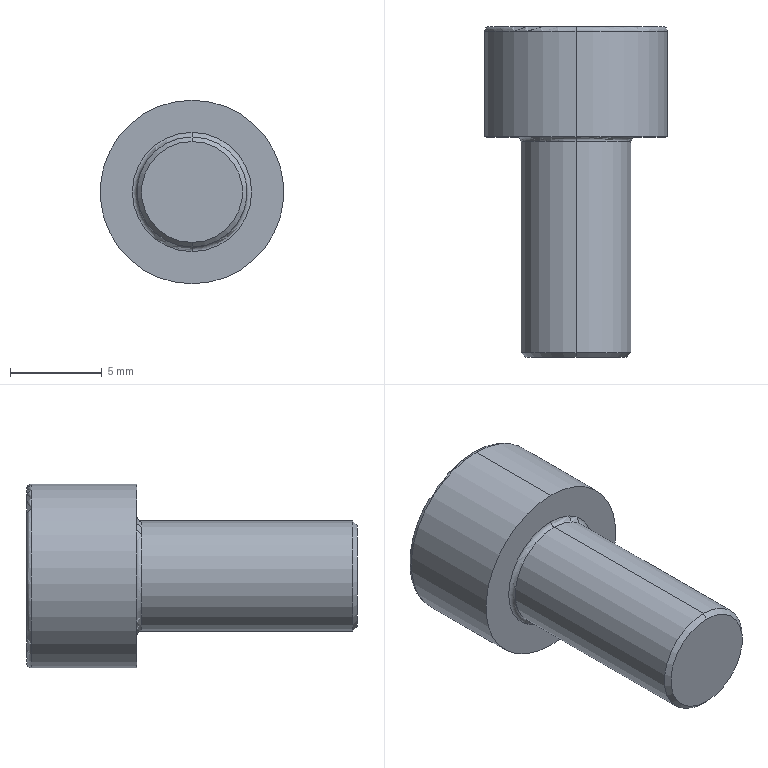Part | STEP file | 1 solid | 20 faces | box 10 x 18 x 10 mm | volume 744.847 mm3 | plane 10 | torus 4 | cylinder 4 | cone 2 | commonest cylinder face diameters 6 x2 10 x2
STEP:
#1=CARTESIAN_POINT('',(0.,-12.,-2.75));
#2=VERTEX_POINT('',#1);
#3=CARTESIAN_POINT('',(0.,-12.,2.75));
#4=VERTEX_POINT('',#3);
#5=CARTESIAN_POINT('',(0.,-12.,0.));
#6=DIRECTION('',(0.,-1.,0.));
#7=DIRECTION('',(0.,0.,-1.));
#8=AXIS2_PLACEMENT_3D('',#5,#6,#7);
#9=CIRCLE('',#8,2.75);
#10=EDGE_CURVE('',#2,#4,#9,.T.);
#11=ORIENTED_EDGE('',*,*,#10,.F.);
#12=CARTESIAN_POINT('',(0.,-11.75,-3.));
#13=VERTEX_POINT('',#12);
#14=CARTESIAN_POINT('',(0.,-12.,-2.75));
#15=DIRECTION('',(0.,0.7071,-0.7071));
#16=VECTOR('',#15,1000.);
#17=LINE('',#14,#16);
#18=EDGE_CURVE('',#2,#13,#17,.T.);
#19=ORIENTED_EDGE('',*,*,#18,.T.);
#20=CARTESIAN_POINT('',(0.,-11.75,3.));
#21=VERTEX_POINT('',#20);
#22=CARTESIAN_POINT('',(0.,-11.75,0.));
#23=DIRECTION('',(0.,1.,0.));
#24=DIRECTION('',(0.,0.,-1.));
#25=AXIS2_PLACEMENT_3D('',#22,#23,#24);
#26=CIRCLE('',#25,3.);
#27=EDGE_CURVE('',#21,#13,#26,.T.);
#28=ORIENTED_EDGE('',*,*,#27,.F.);
#29=CARTESIAN_POINT('',(0.,-12.,2.75));
#30=DIRECTION('',(0.,0.7071,0.7071));
#31=VECTOR('',#30,1000.);
#32=LINE('',#29,#31);
#33=EDGE_CURVE('',#4,#21,#32,.T.);
#34=ORIENTED_EDGE('',*,*,#33,.F.);
#35=EDGE_LOOP('',(#11,#19,#28,#34));
#36=FACE_OUTER_BOUND('',#35,.T.);
#37=CARTESIAN_POINT('',(0.,-12.,0.));
#38=DIRECTION('',(0.,1.,0.));
#39=DIRECTION('',(0.,0.,1.));
#40=AXIS2_PLACEMENT_3D('',#37,#38,#39);
#41=CONICAL_SURFACE('',#40,2.75,0.7854);
#42=ADVANCED_FACE('',(#36),#41,.T.);
#43=CARTESIAN_POINT('',(0.,5.75,-5.));
#44=VERTEX_POINT('',#43);
#45=CARTESIAN_POINT('',(0.,5.75,5.));
#46=VERTEX_POINT('',#45);
#47=CARTESIAN_POINT('',(0.,5.75,0.));
#48=DIRECTION('',(0.,-1.,0.));
#49=DIRECTION('',(0.,0.,1.));
#50=AXIS2_PLACEMENT_3D('',#47,#48,#49);
#51=CIRCLE('',#50,5.);
#52=EDGE_CURVE('',#44,#46,#51,.T.);
#53=ORIENTED_EDGE('',*,*,#52,.F.);
#54=CARTESIAN_POINT('',(0.,6.,-4.75));
#55=VERTEX_POINT('',#54);
#56=CARTESIAN_POINT('',(0.,5.75,-4.75));
#57=DIRECTION('',(1.,0.,0.));
#58=DIRECTION('',(0.,0.,-1.));
#59=AXIS2_PLACEMENT_3D('',#56,#57,#58);
#60=CIRCLE('',#59,0.25);
#61=EDGE_CURVE('',#44,#55,#60,.T.);
#62=ORIENTED_EDGE('',*,*,#61,.T.);
#63=CARTESIAN_POINT('',(0.,6.,4.75));
#64=VERTEX_POINT('',#63);
#65=CARTESIAN_POINT('',(0.,6.,0.));
#66=DIRECTION('',(0.,1.,0.));
#67=DIRECTION('',(0.,0.,1.));
#68=AXIS2_PLACEMENT_3D('',#65,#66,#67);
#69=CIRCLE('',#68,4.75);
#70=EDGE_CURVE('',#64,#55,#69,.T.);
#71=ORIENTED_EDGE('',*,*,#70,.F.);
#72=CARTESIAN_POINT('',(0.,5.75,4.75));
#73=DIRECTION('',(-1.,0.,0.));
#74=DIRECTION('',(0.,0.,1.));
#75=AXIS2_PLACEMENT_3D('',#72,#73,#74);
#76=CIRCLE('',#75,0.25);
#77=EDGE_CURVE('',#46,#64,#76,.T.);
#78=ORIENTED_EDGE('',*,*,#77,.F.);
#79=EDGE_LOOP('',(#53,#62,#71,#78));
#80=FACE_OUTER_BOUND('',#79,.T.);
#81=CARTESIAN_POINT('',(0.,5.75,0.));
#82=DIRECTION('',(0.,1.,0.));
#83=DIRECTION('',(0.,0.,1.));
#84=AXIS2_PLACEMENT_3D('',#81,#82,#83);
#85=TOROIDAL_SURFACE('',#84,4.75,0.25);
#86=ADVANCED_FACE('',(#80),#85,.T.);
#87=CARTESIAN_POINT('',(0.,-0.25,3.));
#88=VERTEX_POINT('',#87);
#89=CARTESIAN_POINT('',(0.,-0.25,-3.));
#90=VERTEX_POINT('',#89);
#91=CARTESIAN_POINT('',(0.,-0.25,0.));
#92=DIRECTION('',(0.,-1.,0.));
#93=DIRECTION('',(0.,0.,-1.));
#94=AXIS2_PLACEMENT_3D('',#91,#92,#93);
#95=CIRCLE('',#94,3.);
#96=EDGE_CURVE('',#88,#90,#95,.T.);
#97=ORIENTED_EDGE('',*,*,#96,.F.);
#98=CARTESIAN_POINT('',(0.,0.,3.25));
#99=VERTEX_POINT('',#98);
#100=CARTESIAN_POINT('',(0.,-0.25,3.25));
#101=DIRECTION('',(1.,0.,0.));
#102=DIRECTION('',(0.,0.,-1.));
#103=AXIS2_PLACEMENT_3D('',#100,#101,#102);
#104=CIRCLE('',#103,0.25);
#105=EDGE_CURVE('',#88,#99,#104,.T.);
#106=ORIENTED_EDGE('',*,*,#105,.T.);
#107=CARTESIAN_POINT('',(0.,0.,-3.25));
#108=VERTEX_POINT('',#107);
#109=CARTESIAN_POINT('',(0.,0.,0.));
#110=DIRECTION('',(0.,1.,0.));
#111=DIRECTION('',(0.,0.,-1.));
#112=AXIS2_PLACEMENT_3D('',#109,#110,#111);
#113=CIRCLE('',#112,3.25);
#114=EDGE_CURVE('',#108,#99,#113,.T.);
#115=ORIENTED_EDGE('',*,*,#114,.F.);
#116=CARTESIAN_POINT('',(0.,-0.25,-3.25));
#117=DIRECTION('',(-1.,0.,0.));
#118=DIRECTION('',(0.,0.,1.));
#119=AXIS2_PLACEMENT_3D('',#116,#117,#118);
#120=CIRCLE('',#119,0.25);
#121=EDGE_CURVE('',#90,#108,#120,.T.);
#122=ORIENTED_EDGE('',*,*,#121,.F.);
#123=EDGE_LOOP('',(#97,#106,#115,#122));
#124=FACE_OUTER_BOUND('',#123,.T.);
#125=CARTESIAN_POINT('',(0.,-0.25,0.));
#126=DIRECTION('',(0.,-1.,0.));
#127=DIRECTION('',(0.,0.,-1.));
#128=AXIS2_PLACEMENT_3D('',#125,#126,#127);
#129=TOROIDAL_SURFACE('',#128,3.25,0.25);
#130=ADVANCED_FACE('',(#124),#129,.F.);
#131=CARTESIAN_POINT('',(0.,-0.25,0.));
#132=DIRECTION('',(0.,-1.,0.));
#133=DIRECTION('',(0.,0.,-1.));
#134=AXIS2_PLACEMENT_3D('',#131,#132,#133);
#135=CIRCLE('',#134,3.);
#136=EDGE_CURVE('',#90,#88,#135,.T.);
#137=ORIENTED_EDGE('',*,*,#136,.T.);
#138=CARTESIAN_POINT('',(0.,0.,3.));
#139=DIRECTION('',(0.,-1.,0.));
#140=VECTOR('',#139,1000.);
#141=LINE('',#138,#140);
#142=EDGE_CURVE('',#88,#21,#141,.T.);
#143=ORIENTED_EDGE('',*,*,#142,.T.);
#144=ORIENTED_EDGE('',*,*,#27,.T.);
#145=CARTESIAN_POINT('',(0.,0.,-3.));
#146=DIRECTION('',(0.,-1.,0.));
#147=VECTOR('',#146,1000.);
#148=LINE('',#145,#147);
#149=EDGE_CURVE('',#90,#13,#148,.T.);
#150=ORIENTED_EDGE('',*,*,#149,.F.);
#151=EDGE_LOOP('',(#137,#143,#144,#150));
#152=FACE_OUTER_BOUND('',#151,.T.);
#153=CARTESIAN_POINT('',(0.,0.,0.));
#154=DIRECTION('',(0.,-1.,0.));
#155=DIRECTION('',(0.,0.,-1.));
#156=AXIS2_PLACEMENT_3D('',#153,#154,#155);
#157=CYLINDRICAL_SURFACE('',#156,3.);
#158=ADVANCED_FACE('',(#152),#157,.T.);
#159=ORIENTED_EDGE('',*,*,#52,.T.);
#160=CARTESIAN_POINT('',(0.,0.,5.));
#161=VERTEX_POINT('',#160);
#162=CARTESIAN_POINT('',(0.,0.,5.));
#163=DIRECTION('',(0.,-1.,0.));
#164=VECTOR('',#163,1000.);
#165=LINE('',#162,#164);
#166=EDGE_CURVE('',#46,#161,#165,.T.);
#167=ORIENTED_EDGE('',*,*,#166,.T.);
#168=CARTESIAN_POINT('',(0.,0.,-5.));
#169=VERTEX_POINT('',#168);
#170=CARTESIAN_POINT('',(0.,0.,0.));
#171=DIRECTION('',(0.,-1.,0.));
#172=DIRECTION('',(0.,0.,-1.));
#173=AXIS2_PLACEMENT_3D('',#170,#171,#172);
#174=CIRCLE('',#173,5.);
#175=EDGE_CURVE('',#169,#161,#174,.T.);
#176=ORIENTED_EDGE('',*,*,#175,.F.);
#177=CARTESIAN_POINT('',(0.,0.,-5.));
#178=DIRECTION('',(0.,-1.,0.));
#179=VECTOR('',#178,1000.);
#180=LINE('',#177,#179);
#181=EDGE_CURVE('',#44,#169,#180,.T.);
#182=ORIENTED_EDGE('',*,*,#181,.F.);
#183=EDGE_LOOP('',(#159,#167,#176,#182));
#184=FACE_OUTER_BOUND('',#183,.T.);
#185=CARTESIAN_POINT('',(0.,0.,0.));
#186=DIRECTION('',(0.,-1.,0.));
#187=DIRECTION('',(0.,0.,-1.));
#188=AXIS2_PLACEMENT_3D('',#185,#186,#187);
#189=CYLINDRICAL_SURFACE('',#188,5.);
#190=ADVANCED_FACE('',(#184),#189,.T.);
#191=ORIENTED_EDGE('',*,*,#70,.T.);
#192=CARTESIAN_POINT('',(0.,6.,0.));
#193=DIRECTION('',(0.,1.,0.));
#194=DIRECTION('',(0.,0.,1.));
#195=AXIS2_PLACEMENT_3D('',#192,#193,#194);
#196=CIRCLE('',#195,4.75);
#197=EDGE_CURVE('',#55,#64,#196,.T.);
#198=ORIENTED_EDGE('',*,*,#197,.T.);
#199=EDGE_LOOP('',(#191,#198));
#200=FACE_OUTER_BOUND('',#199,.T.);
#201=CARTESIAN_POINT('',(0.,6.,-2.887));
#202=VERTEX_POINT('',#201);
#203=CARTESIAN_POINT('',(-2.5,6.,-1.443));
#204=VERTEX_POINT('',#203);
#205=CARTESIAN_POINT('',(0.,6.,-2.887));
#206=DIRECTION('',(-0.866,0.,0.5));
#207=VECTOR('',#206,1000.);
#208=LINE('',#205,#207);
#209=EDGE_CURVE('',#202,#204,#208,.T.);
#210=ORIENTED_EDGE('',*,*,#209,.F.);
#211=CARTESIAN_POINT('',(2.5,6.,-1.443));
#212=VERTEX_POINT('',#211);
#213=CARTESIAN_POINT('',(2.5,6.,-1.443));
#214=DIRECTION('',(-0.866,0.,-0.5));
#215=VECTOR('',#214,1000.);
#216=LINE('',#213,#215);
#217=EDGE_CURVE('',#212,#202,#216,.T.);
#218=ORIENTED_EDGE('',*,*,#217,.F.);
#219=CARTESIAN_POINT('',(2.5,6.,1.443));
#220=VERTEX_POINT('',#219);
#221=CARTESIAN_POINT('',(2.5,6.,1.443));
#222=DIRECTION('',(0.,0.,-1.));
#223=VECTOR('',#222,1000.);
#224=LINE('',#221,#223);
#225=EDGE_CURVE('',#220,#212,#224,.T.);
#226=ORIENTED_EDGE('',*,*,#225,.F.);
#227=CARTESIAN_POINT('',(0.,6.,2.887));
#228=VERTEX_POINT('',#227);
#229=CARTESIAN_POINT('',(0.,6.,2.887));
#230=DIRECTION('',(0.866,0.,-0.5));
#231=VECTOR('',#230,1000.);
#232=LINE('',#229,#231);
#233=EDGE_CURVE('',#228,#220,#232,.T.);
#234=ORIENTED_EDGE('',*,*,#233,.F.);
#235=CARTESIAN_POINT('',(-2.5,6.,1.443));
#236=VERTEX_POINT('',#235);
#237=CARTESIAN_POINT('',(-2.5,6.,1.443));
#238=DIRECTION('',(0.866,0.,0.5));
#239=VECTOR('',#238,1000.);
#240=LINE('',#237,#239);
#241=EDGE_CURVE('',#236,#228,#240,.T.);
#242=ORIENTED_EDGE('',*,*,#241,.F.);
#243=CARTESIAN_POINT('',(-2.5,6.,-1.443));
#244=DIRECTION('',(0.,0.,1.));
#245=VECTOR('',#244,1000.);
#246=LINE('',#243,#245);
#247=EDGE_CURVE('',#204,#236,#246,.T.);
#248=ORIENTED_EDGE('',*,*,#247,.F.);
#249=EDGE_LOOP('',(#210,#218,#226,#234,#242,#248));
#250=FACE_BOUND('',#249,.T.);
#251=CARTESIAN_POINT('',(0.,6.,0.));
#252=DIRECTION('',(0.,1.,0.));
#253=DIRECTION('',(0.,0.,1.));
#254=AXIS2_PLACEMENT_3D('',#251,#252,#253);
#255=PLANE('',#254);
#256=ADVANCED_FACE('',(#200,#250),#255,.T.);
#257=ORIENTED_EDGE('',*,*,#166,.F.);
#258=CARTESIAN_POINT('',(0.,5.75,0.));
#259=DIRECTION('',(0.,-1.,0.));
#260=DIRECTION('',(0.,0.,1.));
#261=AXIS2_PLACEMENT_3D('',#258,#259,#260);
#262=CIRCLE('',#261,5.);
#263=EDGE_CURVE('',#46,#44,#262,.T.);
#264=ORIENTED_EDGE('',*,*,#263,.T.);
#265=ORIENTED_EDGE('',*,*,#181,.T.);
#266=CARTESIAN_POINT('',(0.,0.,0.));
#267=DIRECTION('',(0.,-1.,0.));
#268=DIRECTION('',(0.,0.,-1.));
#269=AXIS2_PLACEMENT_3D('',#266,#267,#268);
#270=CIRCLE('',#269,5.);
#271=EDGE_CURVE('',#161,#169,#270,.T.);
#272=ORIENTED_EDGE('',*,*,#271,.F.);
#273=EDGE_LOOP('',(#257,#264,#265,#272));
#274=FACE_OUTER_BOUND('',#273,.T.);
#275=CARTESIAN_POINT('',(0.,0.,0.));
#276=DIRECTION('',(0.,-1.,0.));
#277=DIRECTION('',(0.,0.,-1.));
#278=AXIS2_PLACEMENT_3D('',#275,#276,#277);
#279=CYLINDRICAL_SURFACE('',#278,5.);
#280=ADVANCED_FACE('',(#274),#279,.T.);
#281=ORIENTED_EDGE('',*,*,#114,.T.);
#282=CARTESIAN_POINT('',(0.,0.,0.));
#283=DIRECTION('',(0.,1.,0.));
#284=DIRECTION('',(0.,0.,-1.));
#285=AXIS2_PLACEMENT_3D('',#282,#283,#284);
#286=CIRCLE('',#285,3.25);
#287=EDGE_CURVE('',#99,#108,#286,.T.);
#288=ORIENTED_EDGE('',*,*,#287,.T.);
#289=EDGE_LOOP('',(#281,#288));
#290=FACE_BOUND('',#289,.T.);
#291=ORIENTED_EDGE('',*,*,#175,.T.);
#292=ORIENTED_EDGE('',*,*,#271,.T.);
#293=EDGE_LOOP('',(#291,#292));
#294=FACE_OUTER_BOUND('',#293,.T.);
#295=CARTESIAN_POINT('',(5.,0.,0.));
#296=DIRECTION('',(0.,-1.,0.));
#297=DIRECTION('',(0.,0.,-1.));
#298=AXIS2_PLACEMENT_3D('',#295,#296,#297);
#299=PLANE('',#298);
#300=ADVANCED_FACE('',(#290,#294),#299,.T.);
#301=ORIENTED_EDGE('',*,*,#142,.F.);
#302=ORIENTED_EDGE('',*,*,#96,.T.);
#303=ORIENTED_EDGE('',*,*,#149,.T.);
#304=CARTESIAN_POINT('',(0.,-11.75,0.));
#305=DIRECTION('',(0.,1.,0.));
#306=DIRECTION('',(0.,0.,-1.));
#307=AXIS2_PLACEMENT_3D('',#304,#305,#306);
#308=CIRCLE('',#307,3.);
#309=EDGE_CURVE('',#13,#21,#308,.T.);
#310=ORIENTED_EDGE('',*,*,#309,.T.);
#311=EDGE_LOOP('',(#301,#302,#303,#310));
#312=FACE_OUTER_BOUND('',#311,.T.);
#313=CARTESIAN_POINT('',(0.,0.,0.));
#314=DIRECTION('',(0.,-1.,0.));
#315=DIRECTION('',(0.,0.,-1.));
#316=AXIS2_PLACEMENT_3D('',#313,#314,#315);
#317=CYLINDRICAL_SURFACE('',#316,3.);
#318=ADVANCED_FACE('',(#312),#317,.T.);
#319=CARTESIAN_POINT('',(0.,-12.,0.));
#320=DIRECTION('',(0.,-1.,0.));
#321=DIRECTION('',(0.,0.,-1.));
#322=AXIS2_PLACEMENT_3D('',#319,#320,#321);
#323=CIRCLE('',#322,2.75);
#324=EDGE_CURVE('',#4,#2,#323,.T.);
#325=ORIENTED_EDGE('',*,*,#324,.T.);
#326=ORIENTED_EDGE('',*,*,#10,.T.);
#327=EDGE_LOOP('',(#325,#326));
#328=FACE_OUTER_BOUND('',#327,.T.);
#329=CARTESIAN_POINT('',(3.,-12.,0.));
#330=DIRECTION('',(0.,-1.,0.));
#331=DIRECTION('',(0.,0.,-1.));
#332=AXIS2_PLACEMENT_3D('',#329,#330,#331);
#333=PLANE('',#332);
#334=ADVANCED_FACE('',(#328),#333,.T.);
#335=ORIENTED_EDGE('',*,*,#209,.T.);
#336=CARTESIAN_POINT('',(-2.5,3.,-1.443));
#337=VERTEX_POINT('',#336);
#338=CARTESIAN_POINT('',(-2.5,3.,-1.443));
#339=DIRECTION('',(0.,1.,0.));
#340=VECTOR('',#339,1000.);
#341=LINE('',#338,#340);
#342=EDGE_CURVE('',#337,#204,#341,.T.);
#343=ORIENTED_EDGE('',*,*,#342,.F.);
#344=CARTESIAN_POINT('',(0.,3.,-2.887));
#345=VERTEX_POINT('',#344);
#346=CARTESIAN_POINT('',(0.,3.,-2.887));
#347=DIRECTION('',(-0.866,0.,0.5));
#348=VECTOR('',#347,1000.);
#349=LINE('',#346,#348);
#350=EDGE_CURVE('',#345,#337,#349,.T.);
#351=ORIENTED_EDGE('',*,*,#350,.F.);
#352=CARTESIAN_POINT('',(0.,3.,-2.887));
#353=DIRECTION('',(0.,1.,0.));
#354=VECTOR('',#353,1000.);
#355=LINE('',#352,#354);
#356=EDGE_CURVE('',#345,#202,#355,.T.);
#357=ORIENTED_EDGE('',*,*,#356,.T.);
#358=EDGE_LOOP('',(#335,#343,#351,#357));
#359=FACE_OUTER_BOUND('',#358,.T.);
#360=CARTESIAN_POINT('',(0.,3.,-2.887));
#361=DIRECTION('',(-0.5,0.,-0.866));
#362=DIRECTION('',(-0.866,0.,0.5));
#363=AXIS2_PLACEMENT_3D('',#360,#361,#362);
#364=PLANE('',#363);
#365=ADVANCED_FACE('',(#359),#364,.F.);
#366=ORIENTED_EDGE('',*,*,#217,.T.);
#367=ORIENTED_EDGE('',*,*,#356,.F.);
#368=CARTESIAN_POINT('',(2.5,3.,-1.443));
#369=VERTEX_POINT('',#368);
#370=CARTESIAN_POINT('',(2.5,3.,-1.443));
#371=DIRECTION('',(-0.866,0.,-0.5));
#372=VECTOR('',#371,1000.);
#373=LINE('',#370,#372);
#374=EDGE_CURVE('',#369,#345,#373,.T.);
#375=ORIENTED_EDGE('',*,*,#374,.F.);
#376=CARTESIAN_POINT('',(2.5,3.,-1.443));
#377=DIRECTION('',(0.,1.,0.));
#378=VECTOR('',#377,1000.);
#379=LINE('',#376,#378);
#380=EDGE_CURVE('',#369,#212,#379,.T.);
#381=ORIENTED_EDGE('',*,*,#380,.T.);
#382=EDGE_LOOP('',(#366,#367,#375,#381));
#383=FACE_OUTER_BOUND('',#382,.T.);
#384=CARTESIAN_POINT('',(2.5,3.,-1.443));
#385=DIRECTION('',(0.5,0.,-0.866));
#386=DIRECTION('',(-0.866,0.,-0.5));
#387=AXIS2_PLACEMENT_3D('',#384,#385,#386);
#388=PLANE('',#387);
#389=ADVANCED_FACE('',(#383),#388,.F.);
#390=ORIENTED_EDGE('',*,*,#225,.T.);
#391=ORIENTED_EDGE('',*,*,#380,.F.);
#392=CARTESIAN_POINT('',(2.5,3.,1.443));
#393=VERTEX_POINT('',#392);
#394=CARTESIAN_POINT('',(2.5,3.,1.443));
#395=DIRECTION('',(0.,0.,-1.));
#396=VECTOR('',#395,1000.);
#397=LINE('',#394,#396);
#398=EDGE_CURVE('',#393,#369,#397,.T.);
#399=ORIENTED_EDGE('',*,*,#398,.F.);
#400=CARTESIAN_POINT('',(2.5,3.,1.443));
#401=DIRECTION('',(0.,1.,0.));
#402=VECTOR('',#401,1000.);
#403=LINE('',#400,#402);
#404=EDGE_CURVE('',#393,#220,#403,.T.);
#405=ORIENTED_EDGE('',*,*,#404,.T.);
#406=EDGE_LOOP('',(#390,#391,#399,#405));
#407=FACE_OUTER_BOUND('',#406,.T.);
#408=CARTESIAN_POINT('',(2.5,3.,1.443));
#409=DIRECTION('',(1.,0.,0.));
#410=DIRECTION('',(0.,0.,-1.));
#411=AXIS2_PLACEMENT_3D('',#408,#409,#410);
#412=PLANE('',#411);
#413=ADVANCED_FACE('',(#407),#412,.F.);
#414=ORIENTED_EDGE('',*,*,#233,.T.);
#415=ORIENTED_EDGE('',*,*,#404,.F.);
#416=CARTESIAN_POINT('',(0.,3.,2.887));
#417=VERTEX_POINT('',#416);
#418=CARTESIAN_POINT('',(0.,3.,2.887));
#419=DIRECTION('',(0.866,0.,-0.5));
#420=VECTOR('',#419,1000.);
#421=LINE('',#418,#420);
#422=EDGE_CURVE('',#417,#393,#421,.T.);
#423=ORIENTED_EDGE('',*,*,#422,.F.);
#424=CARTESIAN_POINT('',(0.,3.,2.887));
#425=DIRECTION('',(0.,1.,0.));
#426=VECTOR('',#425,1000.);
#427=LINE('',#424,#426);
#428=EDGE_CURVE('',#417,#228,#427,.T.);
#429=ORIENTED_EDGE('',*,*,#428,.T.);
#430=EDGE_LOOP('',(#414,#415,#423,#429));
#431=FACE_OUTER_BOUND('',#430,.T.);
#432=CARTESIAN_POINT('',(0.,3.,2.887));
#433=DIRECTION('',(0.5,0.,0.866));
#434=DIRECTION('',(0.866,0.,-0.5));
#435=AXIS2_PLACEMENT_3D('',#432,#433,#434);
#436=PLANE('',#435);
#437=ADVANCED_FACE('',(#431),#436,.F.);
#438=ORIENTED_EDGE('',*,*,#241,.T.);
#439=ORIENTED_EDGE('',*,*,#428,.F.);
#440=CARTESIAN_POINT('',(-2.5,3.,1.443));
#441=VERTEX_POINT('',#440);
#442=CARTESIAN_POINT('',(-2.5,3.,1.443));
#443=DIRECTION('',(0.866,0.,0.5));
#444=VECTOR('',#443,1000.);
#445=LINE('',#442,#444);
#446=EDGE_CURVE('',#441,#417,#445,.T.);
#447=ORIENTED_EDGE('',*,*,#446,.F.);
#448=CARTESIAN_POINT('',(-2.5,3.,1.443));
#449=DIRECTION('',(0.,1.,0.));
#450=VECTOR('',#449,1000.);
#451=LINE('',#448,#450);
#452=EDGE_CURVE('',#441,#236,#451,.T.);
#453=ORIENTED_EDGE('',*,*,#452,.T.);
#454=EDGE_LOOP('',(#438,#439,#447,#453));
#455=FACE_OUTER_BOUND('',#454,.T.);
#456=CARTESIAN_POINT('',(-2.5,3.,1.443));
#457=DIRECTION('',(-0.5,0.,0.866));
#458=DIRECTION('',(0.866,0.,0.5));
#459=AXIS2_PLACEMENT_3D('',#456,#457,#458);
#460=PLANE('',#459);
#461=ADVANCED_FACE('',(#455),#460,.F.);
#462=ORIENTED_EDGE('',*,*,#247,.T.);
#463=ORIENTED_EDGE('',*,*,#452,.F.);
#464=CARTESIAN_POINT('',(-2.5,3.,-1.443));
#465=DIRECTION('',(0.,0.,1.));
#466=VECTOR('',#465,1000.);
#467=LINE('',#464,#466);
#468=EDGE_CURVE('',#337,#441,#467,.T.);
#469=ORIENTED_EDGE('',*,*,#468,.F.);
#470=ORIENTED_EDGE('',*,*,#342,.T.);
#471=EDGE_LOOP('',(#462,#463,#469,#470));
#472=FACE_OUTER_BOUND('',#471,.T.);
#473=CARTESIAN_POINT('',(-2.5,3.,-1.443));
#474=DIRECTION('',(-1.,0.,0.));
#475=DIRECTION('',(0.,0.,1.));
#476=AXIS2_PLACEMENT_3D('',#473,#474,#475);
#477=PLANE('',#476);
#478=ADVANCED_FACE('',(#472),#477,.F.);
#479=ORIENTED_EDGE('',*,*,#350,.T.);
#480=ORIENTED_EDGE('',*,*,#468,.T.);
#481=ORIENTED_EDGE('',*,*,#446,.T.);
#482=ORIENTED_EDGE('',*,*,#422,.T.);
#483=ORIENTED_EDGE('',*,*,#398,.T.);
#484=ORIENTED_EDGE('',*,*,#374,.T.);
#485=EDGE_LOOP('',(#479,#480,#481,#482,#483,#484));
#486=FACE_OUTER_BOUND('',#485,.T.);
#487=CARTESIAN_POINT('',(0.,3.,0.));
#488=DIRECTION('',(0.,1.,0.));
#489=DIRECTION('',(0.,0.,1.));
#490=AXIS2_PLACEMENT_3D('',#487,#488,#489);
#491=PLANE('',#490);
#492=ADVANCED_FACE('',(#486),#491,.T.);
#493=ORIENTED_EDGE('',*,*,#105,.F.);
#494=ORIENTED_EDGE('',*,*,#136,.F.);
#495=ORIENTED_EDGE('',*,*,#121,.T.);
#496=ORIENTED_EDGE('',*,*,#287,.F.);
#497=EDGE_LOOP('',(#493,#494,#495,#496));
#498=FACE_OUTER_BOUND('',#497,.T.);
#499=CARTESIAN_POINT('',(0.,-0.25,0.));
#500=DIRECTION('',(0.,-1.,0.));
#501=DIRECTION('',(0.,0.,-1.));
#502=AXIS2_PLACEMENT_3D('',#499,#500,#501);
#503=TOROIDAL_SURFACE('',#502,3.25,0.25);
#504=ADVANCED_FACE('',(#498),#503,.F.);
#505=ORIENTED_EDGE('',*,*,#61,.F.);
#506=ORIENTED_EDGE('',*,*,#263,.F.);
#507=ORIENTED_EDGE('',*,*,#77,.T.);
#508=ORIENTED_EDGE('',*,*,#197,.F.);
#509=EDGE_LOOP('',(#505,#506,#507,#508));
#510=FACE_OUTER_BOUND('',#509,.T.);
#511=CARTESIAN_POINT('',(0.,5.75,0.));
#512=DIRECTION('',(0.,1.,0.));
#513=DIRECTION('',(0.,0.,1.));
#514=AXIS2_PLACEMENT_3D('',#511,#512,#513);
#515=TOROIDAL_SURFACE('',#514,4.75,0.25);
#516=ADVANCED_FACE('',(#510),#515,.T.);
#517=ORIENTED_EDGE('',*,*,#18,.F.);
#518=ORIENTED_EDGE('',*,*,#324,.F.);
#519=ORIENTED_EDGE('',*,*,#33,.T.);
#520=ORIENTED_EDGE('',*,*,#309,.F.);
#521=EDGE_LOOP('',(#517,#518,#519,#520));
#522=FACE_OUTER_BOUND('',#521,.T.);
#523=CARTESIAN_POINT('',(0.,-12.,0.));
#524=DIRECTION('',(0.,1.,0.));
#525=DIRECTION('',(0.,0.,1.));
#526=AXIS2_PLACEMENT_3D('',#523,#524,#525);
#527=CONICAL_SURFACE('',#526,2.75,0.7854);
#528=ADVANCED_FACE('',(#522),#527,.T.);
#529=CLOSED_SHELL('',(#42,#86,#130,#158,#190,#256,#280,#300,#318,#334,#365,#389,#413,#437,#461,#478,#492,#504,#516,#528));
#530=MANIFOLD_SOLID_BREP('',#529);
#531=CARTESIAN_POINT('',(0.,0.,0.));
#532=DIRECTION('',(0.,0.,1.));
#533=DIRECTION('',(1.,0.,0.));
#534=AXIS2_PLACEMENT_3D('',#531,#532,#533);
#535=(LENGTH_UNIT()NAMED_UNIT(*)SI_UNIT(.MILLI.,.METRE.));
#536=UNCERTAINTY_MEASURE_WITH_UNIT(LENGTH_MEASURE(0.00001),#535,'','');
#537=(NAMED_UNIT(*)PLANE_ANGLE_UNIT()SI_UNIT($,.RADIAN.));
#538=(NAMED_UNIT(*)SI_UNIT($,.STERADIAN.)SOLID_ANGLE_UNIT());
#539=(GEOMETRIC_REPRESENTATION_CONTEXT(3)GLOBAL_UNCERTAINTY_ASSIGNED_CONTEXT((#536))GLOBAL_UNIT_ASSIGNED_CONTEXT((#535,#537,#538))REPRESENTATION_CONTEXT('',''));
#540=ADVANCED_BREP_SHAPE_REPRESENTATION('',(#530,#534),#539);